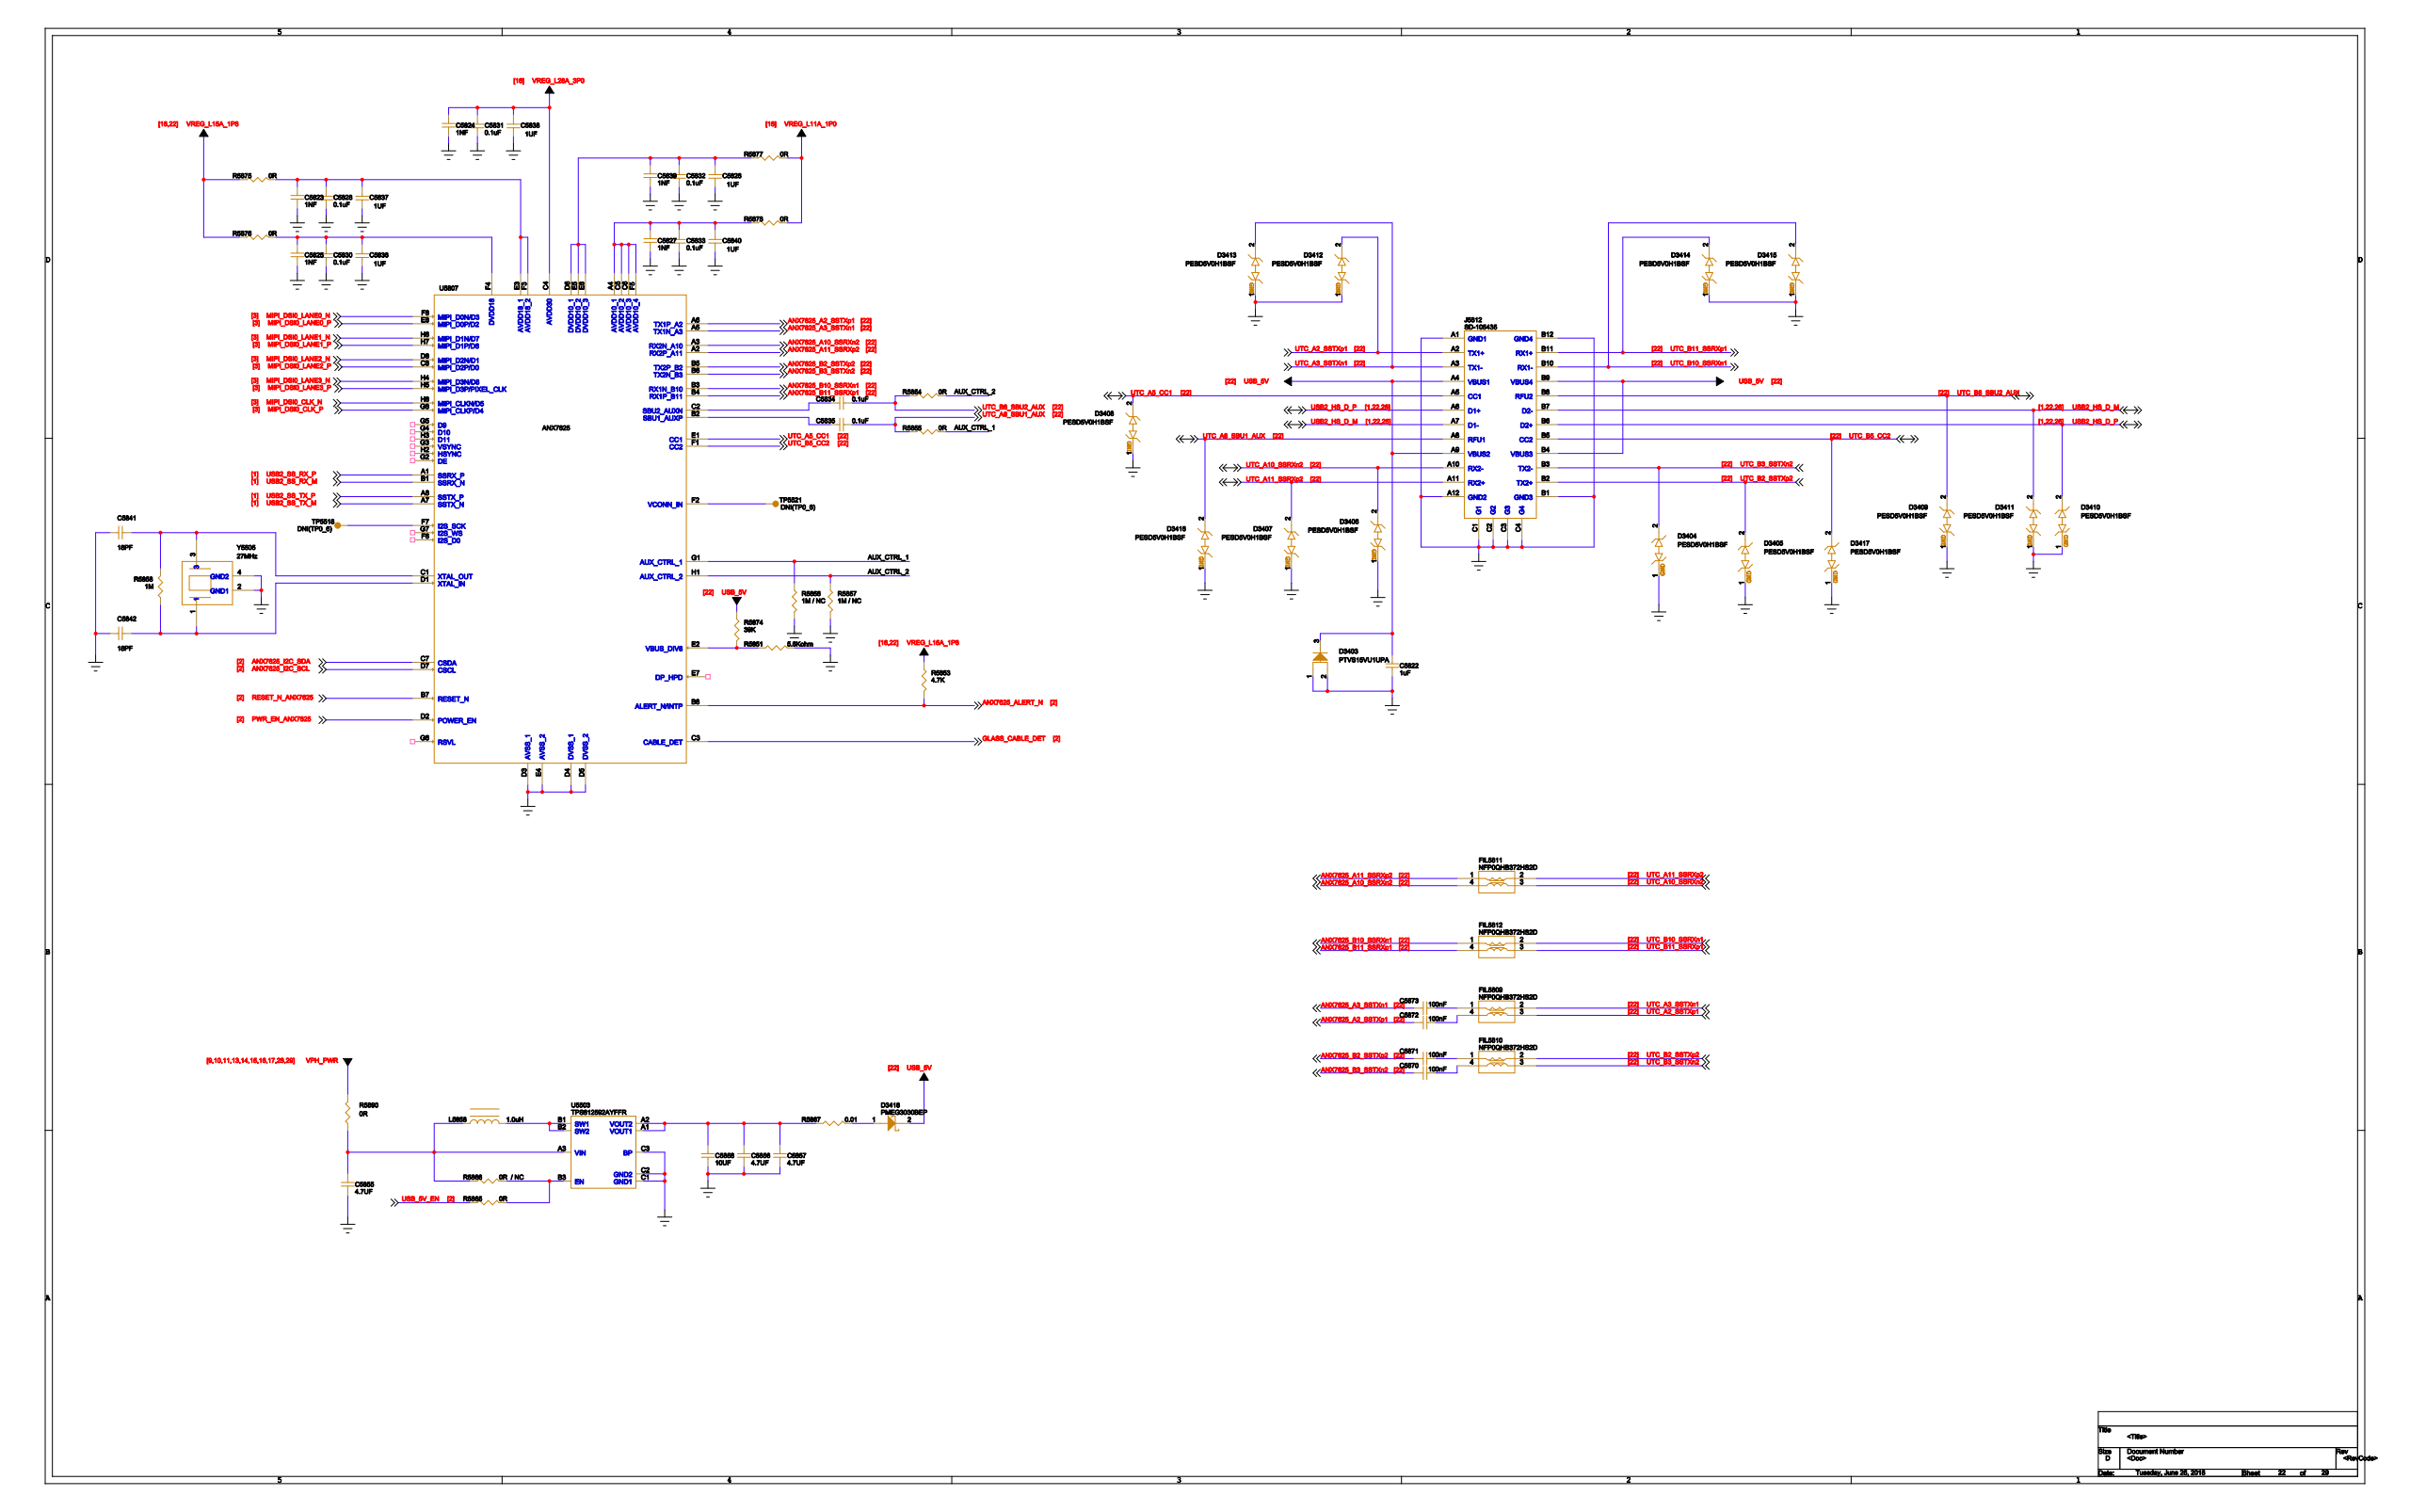Circuit board | Cadence Allegro | 802 parts | 566 nets | one sheet of the schematic
Parts on this sheet (reference | value | footprint):
C5822 | 1UF | C0402
C5823 | 1NF | C0402
C5824 | 1NF | C0402
C5825 | 1NF | C0402
C5826 | 1UF | C0402
C5827 | 1NF | C0402
C5828 | 0.1uF | C0402
C5830 | 0.1uF | C0402
C5831 | 0.1uF | C0402
C5832 | 0.1uF | C0402
C5833 | 0.1uF | C0402
C5834 | 0.1uF | C0402
C5835 | 0.1uF | C0402
C5836 | 1UF | C0402
C5837 | 1UF | C0402
C5838 | 1UF | C0402
C5839 | 1NF | C0402
C5840 | 1UF | C0402
C5841 | 18PF | C0201
C5842 | 18PF | C0201
C5855 | 4.7UF | 0603-BIG
C5856 | 4.7UF | 0603-BIG
C5857 | 4.7UF | 0603-BIG
C5858 | 10uF | 0603-BIG
C5870 | 100NF | C0201
C5871 | 100NF | C0201
C5872 | 100NF | C0201
C5873 | 100NF | C0201
D3403 | PTVS15VU1UPA | DFN2020-3
D3404 | PESD5V0H1BSF | DSN0603-2
D3405 | PESD5V0H1BSF | DSN0603-2
D3406 | PESD5V0H1BSF | DSN0603-2
D3407 | PESD5V0H1BSF | DSN0603-2
D3408 | PESD5V0H1BSF | DSN0603-2
D3409 | PESD5V0H1BSF | DSN0603-2
D3410 | PESD5V0H1BSF | DSN0603-2
D3411 | PESD5V0H1BSF | DSN0603-2
D3412 | PESD5V0H1BSF | DSN0603-2
D3413 | PESD5V0H1BSF | DSN0603-2
D3414 | PESD5V0H1BSF | DSN0603-2
D3415 | PESD5V0H1BSF | DSN0603-2
D3416 | PESD5V0H1BSF | DSN0603-2
D3417 | PESD5V0H1BSF | DSN0603-2
D3418 | PMEG3030BEP | SOD128
FIL5809 | NFP0QHB372HS2D | NFP0QHBXXXHS2X
FIL5810 | NFP0QHB372HS2D | NFP0QHBXXXHS2X
FIL5811 | NFP0QHB372HS2D | NFP0QHBXXXHS2X
FIL5812 | NFP0QHB372HS2D | NFP0QHBXXXHS2X
J5812 | SD-105435 | USB_SD-105435
L5858 | 1.0uH | L2520_TFM252008GHM
R5851 | 5.6Kohm | R0201
R5853 | 4.7K | R0201
R5854 | 0R | R0603
R5855 | 0R | R0603
R5856 | 1M / NC | R0201
R5857 | 1M / NC | R0201
R5858 | 1M | R0201
R5865 | 0R | R0603
R5866 | 0R  / NC | R0603
R5867 | 0.01 | R0603
R5874 | 39K | R0201
R5875 | 0R | R0603
R5876 | 0R | R0603
R5877 | 0R | R0603
R5878 | 0R | R0603
R5890 | 0R | R0603
TP5518 | DNI(TP0_6) | TP_C0P6
TP5521 | DNI(TP0_6) | TP_C0P6
U5503 | TPS612592AYFFR | DSBGA9_1P206X1P306X0P725_0P4
U5807 | ANX7625 | VFBGA64_4X4X1P04_0P4
Y5505 | 27MHz | TZ1897B
Nets of these parts (net: part-pin ...):
GND: C5822-2 C5823-2 C5824-2 C5825-2 C5826-1 C5827-2 C5828-1 C5830-1 C5831-1 C5832-1 C5833-1 C5836-1 C5837-1 C5838-1 C5839-2 C5840-1 C5841-1 C5842-1 C5855-2 C5856-2 C5857-2 C5858-2 D3403-1 D3403-2 D3404-1 D3405-1 D3406-1 D3407-1 D3408-1 D3409-1 D3410-1 D3411-1 D3412-1 D3413-1 D3414-1 D3415-1 D3416-1 D3417-1 R5851-2 R5856-2 R5857-2 U5503-C1 U5503-C2 U5503-C3 Y5505-2 Y5505-4 J5812-A1 J5812-A12 J5812-B1 J5812-B12 J5812-C1 J5812-C2 J5812-C3 J5812-C4 U5807-D3 U5807-D4 U5807-D5 U5807-E4
N328476: C5823-1 C5828-2 C5837-2 R5875-2 U5807-E3 U5807-F3
N328430: C5825-1 C5830-2 C5836-2 R5876-2 U5807-F4
VREG_L28A_3P0: C5824-1 C5831-2 C5838-2 U5807-C4
N328696: C5826-2 C5832-2 C5839-1 R5877-1 U5807-D6 U5807-E5 U5807-E6
N328714: C5827-1 C5833-2 C5840-2 R5878-1 U5807-A4 U5807-C5 U5807-C6 U5807-F5
UTC_B8_SBU2_AUX: C5834-1 D3409-2 R5854-1 J5812-B8
N333461: C5834-2 U5807-C2
UTC_A8_SBU1_AUX: C5835-1 D3416-2 R5855-1 J5812-A8
N333422: C5835-2 U5807-B2
N406426: C5856-1 C5857-1 C5858-1 R5867-1 U5503-A1 U5503-A2
VPH_PWR: R5890-2
N408606: C5870-1 FIL5810-4
ANX7625_B3_SSTXN2: C5870-2 U5807-B6
N408669: C5871-1 FIL5810-1
ANX7625_B2_SSTXP2: C5871-2 U5807-B5
N408590: C5872-1 FIL5809-4
ANX7625_A2_SSTXP1: C5872-2 U5807-A6
N408124: C5873-1 FIL5809-1
ANX7625_A3_SSTXN1: C5873-2 U5807-A5
UTC_B3_SSTXN2: D3404-2 FIL5810-3 J5812-B3
UTC_B2_SSTXP2: D3405-2 FIL5810-2 J5812-B2
UTC_A10_SSRXN2: D3406-2 FIL5811-3 J5812-A10
UTC_A11_SSRXP2: D3407-2 FIL5811-2 J5812-A11
UTC_A5_CC1: D3408-2 J5812-A5 U5807-E1
USB2_HS_D_P: D3410-2 J5812-A6 J5812-B6
USB2_HS_D_M: D3411-2 J5812-A7 J5812-B7
UTC_A2_SSTXP1: D3412-2 FIL5809-3 J5812-A2
UTC_A3_SSTXN1: D3413-2 FIL5809-2 J5812-A3
UTC_B11_SSRXP1: D3414-2 FIL5812-3 J5812-B11
UTC_B10_SSRXN1: D3415-2 FIL5812-2 J5812-B10
UTC_B5_CC2: D3417-2 J5812-B5 U5807-F1
N406422: D3418-1 R5867-2
USB_5V: C5822-1 D3403-3 D3418-2 R5874-1 J5812-A4 J5812-A9 J5812-B4 J5812-B9
N741509: C5841-2 R5858-1 Y5505-3 U5807-C1
N741527: C5842-2 R5858-2 Y5505-1 U5807-D1
N406042: C5855-1 L5858-1 R5866-1 R5890-1 U5503-A3
VREG_L11A_1P0: R5877-2 R5878-2
ANX7625_A11_SSRXP2: FIL5811-1 U5807-A2
ANX7625_A10_SSRXN2: FIL5811-4 U5807-A3
ANX7625_B10_SSRXN1: FIL5812-1 U5807-B3
ANX7625_B11_SSRXP1: FIL5812-4 U5807-B4
N406102: L5858-2 U5503-B1 U5503-B2
ANX7625_I2C_SDA: U5807-C7
ANX7625_I2C_SCL: U5807-D7
AUX_CTRL_2: R5854-2 R5857-1 U5807-H1
AUX_CTRL_1: R5855-2 R5856-1 U5807-G1
USB_5V_EN: R5865-1
N406074: R5865-2 R5866-2 U5503-B3
VREG_L15A_1P8: R5853-1 R5875-1 R5876-1
N334853: R5851-1 R5874-2 U5807-E2
ANX7625_ALERT_N: R5853-2 U5807-B8
N331707: TP5518-1 U5807-F7
N332817: TP5521-1 U5807-F2
USB2_SS_RX_M: U5807-B1
USB2_SS_RX_P: U5807-A1
USB2_SS_TX_M: U5807-A7
USB2_SS_TX_P: U5807-A8
PWR_EN_ANX7625: U5807-D2
RESET_N_ANX7625: U5807-B7
GLASS_CABLE_DET: U5807-C3
MIPI_DSI0_CLK_N: U5807-H8
MIPI_DSI0_CLK_P: U5807-G8
MIPI_DSI0_LANE0_N: U5807-F8
MIPI_DSI0_LANE0_P: U5807-E8
MIPI_DSI0_LANE1_N: U5807-H6
MIPI_DSI0_LANE1_P: U5807-H7
MIPI_DSI0_LANE2_N: U5807-D8
MIPI_DSI0_LANE2_P: U5807-C8
MIPI_DSI0_LANE3_N: U5807-H4
MIPI_DSI0_LANE3_P: U5807-H5